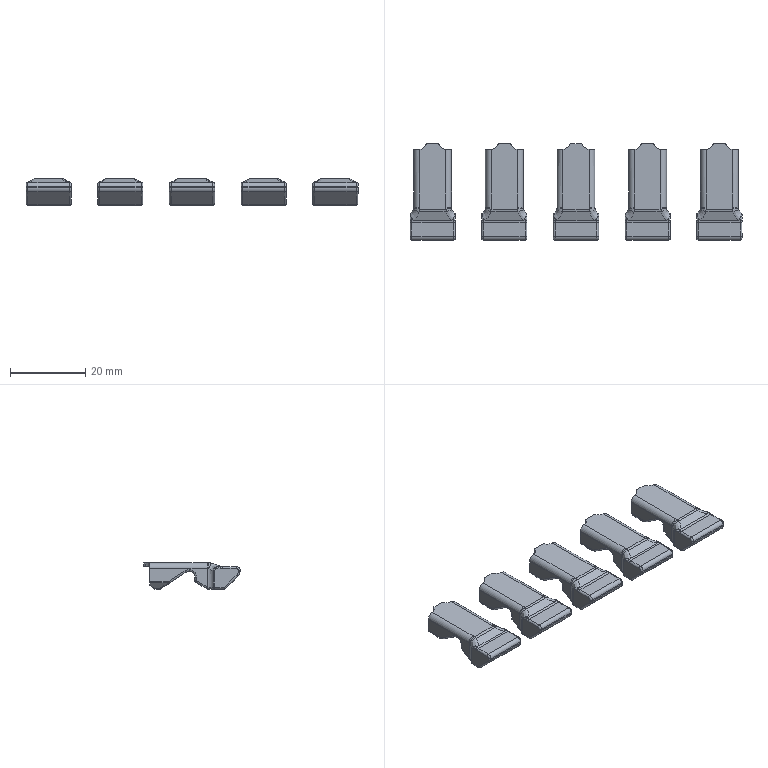Part | 5 solids | 535 faces | box 88 x 25.5 x 7 mm | volume 6261 mm3 | cylinder 225 | plane 105 | spline 70 | torus 65 | sphere 60 | cone 10 | commonest cylinder face diameters 1 x140 4 x30 0.6 x20 3 x20 4.2 x10 2 x5